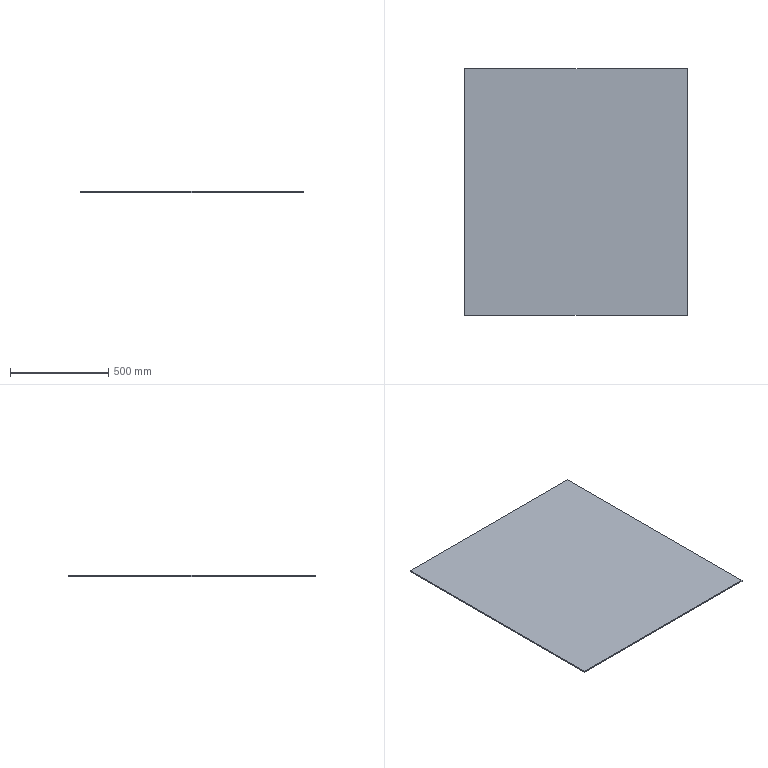Part | SolidWorks | features Extrusion 1 | 1 solid | 6 faces | box 1135 x 1255 x 6 mm | volume 8546550 mm3 | plane 6
STEP:
#1=CARTESIAN_POINT('',(567.5,-627.5,0.));
#2=VERTEX_POINT('',#1);
#3=CARTESIAN_POINT('',(567.5,627.5,0.));
#4=VERTEX_POINT('',#3);
#5=CARTESIAN_POINT('',(567.5,627.5,0.));
#6=DIRECTION('',(0.,1.,0.));
#7=VECTOR('',#6,1000.);
#8=LINE('',#5,#7);
#9=EDGE_CURVE('',#2,#4,#8,.T.);
#10=ORIENTED_EDGE('',*,*,#9,.T.);
#11=CARTESIAN_POINT('',(567.5,627.5,6.));
#12=VERTEX_POINT('',#11);
#13=CARTESIAN_POINT('',(567.5,627.5,6.));
#14=DIRECTION('',(0.,0.,-1.));
#15=VECTOR('',#14,1000.);
#16=LINE('',#13,#15);
#17=EDGE_CURVE('',#12,#4,#16,.T.);
#18=ORIENTED_EDGE('',*,*,#17,.F.);
#19=CARTESIAN_POINT('',(567.5,-627.5,6.));
#20=VERTEX_POINT('',#19);
#21=CARTESIAN_POINT('',(567.5,627.5,6.));
#22=DIRECTION('',(0.,1.,0.));
#23=VECTOR('',#22,1000.);
#24=LINE('',#21,#23);
#25=EDGE_CURVE('',#20,#12,#24,.T.);
#26=ORIENTED_EDGE('',*,*,#25,.F.);
#27=CARTESIAN_POINT('',(567.5,-627.5,6.));
#28=DIRECTION('',(0.,0.,-1.));
#29=VECTOR('',#28,1000.);
#30=LINE('',#27,#29);
#31=EDGE_CURVE('',#20,#2,#30,.T.);
#32=ORIENTED_EDGE('',*,*,#31,.T.);
#33=EDGE_LOOP('',(#10,#18,#26,#32));
#34=FACE_OUTER_BOUND('',#33,.T.);
#35=CARTESIAN_POINT('',(567.5,627.5,6.));
#36=DIRECTION('',(-1.,0.,0.));
#37=DIRECTION('',(0.,-1.,0.));
#38=AXIS2_PLACEMENT_3D('',#35,#36,#37);
#39=PLANE('',#38);
#40=ADVANCED_FACE('',(#34),#39,.F.);
#41=CARTESIAN_POINT('',(-567.5,627.5,0.));
#42=VERTEX_POINT('',#41);
#43=CARTESIAN_POINT('',(-567.5,627.5,0.));
#44=DIRECTION('',(-1.,0.,0.));
#45=VECTOR('',#44,1000.);
#46=LINE('',#43,#45);
#47=EDGE_CURVE('',#4,#42,#46,.T.);
#48=ORIENTED_EDGE('',*,*,#47,.T.);
#49=CARTESIAN_POINT('',(-567.5,627.5,6.));
#50=VERTEX_POINT('',#49);
#51=CARTESIAN_POINT('',(-567.5,627.5,6.));
#52=DIRECTION('',(0.,0.,-1.));
#53=VECTOR('',#52,1000.);
#54=LINE('',#51,#53);
#55=EDGE_CURVE('',#50,#42,#54,.T.);
#56=ORIENTED_EDGE('',*,*,#55,.F.);
#57=CARTESIAN_POINT('',(-567.5,627.5,6.));
#58=DIRECTION('',(-1.,0.,0.));
#59=VECTOR('',#58,1000.);
#60=LINE('',#57,#59);
#61=EDGE_CURVE('',#12,#50,#60,.T.);
#62=ORIENTED_EDGE('',*,*,#61,.F.);
#63=ORIENTED_EDGE('',*,*,#17,.T.);
#64=EDGE_LOOP('',(#48,#56,#62,#63));
#65=FACE_OUTER_BOUND('',#64,.T.);
#66=CARTESIAN_POINT('',(-567.5,627.5,6.));
#67=DIRECTION('',(0.,-1.,0.));
#68=DIRECTION('',(0.,0.,-1.));
#69=AXIS2_PLACEMENT_3D('',#66,#67,#68);
#70=PLANE('',#69);
#71=ADVANCED_FACE('',(#65),#70,.F.);
#72=CARTESIAN_POINT('',(-567.5,-627.5,0.));
#73=VERTEX_POINT('',#72);
#74=CARTESIAN_POINT('',(-567.5,627.5,0.));
#75=DIRECTION('',(0.,-1.,0.));
#76=VECTOR('',#75,1000.);
#77=LINE('',#74,#76);
#78=EDGE_CURVE('',#42,#73,#77,.T.);
#79=ORIENTED_EDGE('',*,*,#78,.T.);
#80=CARTESIAN_POINT('',(-567.5,-627.5,6.));
#81=VERTEX_POINT('',#80);
#82=CARTESIAN_POINT('',(-567.5,-627.5,6.));
#83=DIRECTION('',(0.,0.,-1.));
#84=VECTOR('',#83,1000.);
#85=LINE('',#82,#84);
#86=EDGE_CURVE('',#81,#73,#85,.T.);
#87=ORIENTED_EDGE('',*,*,#86,.F.);
#88=CARTESIAN_POINT('',(-567.5,627.5,6.));
#89=DIRECTION('',(0.,-1.,0.));
#90=VECTOR('',#89,1000.);
#91=LINE('',#88,#90);
#92=EDGE_CURVE('',#50,#81,#91,.T.);
#93=ORIENTED_EDGE('',*,*,#92,.F.);
#94=ORIENTED_EDGE('',*,*,#55,.T.);
#95=EDGE_LOOP('',(#79,#87,#93,#94));
#96=FACE_OUTER_BOUND('',#95,.T.);
#97=CARTESIAN_POINT('',(-567.5,627.5,6.));
#98=DIRECTION('',(1.,0.,0.));
#99=DIRECTION('',(0.,1.,0.));
#100=AXIS2_PLACEMENT_3D('',#97,#98,#99);
#101=PLANE('',#100);
#102=ADVANCED_FACE('',(#96),#101,.F.);
#103=CARTESIAN_POINT('',(-567.5,-627.5,0.));
#104=DIRECTION('',(1.,0.,0.));
#105=VECTOR('',#104,1000.);
#106=LINE('',#103,#105);
#107=EDGE_CURVE('',#73,#2,#106,.T.);
#108=ORIENTED_EDGE('',*,*,#107,.T.);
#109=ORIENTED_EDGE('',*,*,#31,.F.);
#110=CARTESIAN_POINT('',(-567.5,-627.5,6.));
#111=DIRECTION('',(1.,0.,0.));
#112=VECTOR('',#111,1000.);
#113=LINE('',#110,#112);
#114=EDGE_CURVE('',#81,#20,#113,.T.);
#115=ORIENTED_EDGE('',*,*,#114,.F.);
#116=ORIENTED_EDGE('',*,*,#86,.T.);
#117=EDGE_LOOP('',(#108,#109,#115,#116));
#118=FACE_OUTER_BOUND('',#117,.T.);
#119=CARTESIAN_POINT('',(-567.5,-627.5,6.));
#120=DIRECTION('',(0.,1.,0.));
#121=DIRECTION('',(0.,0.,1.));
#122=AXIS2_PLACEMENT_3D('',#119,#120,#121);
#123=PLANE('',#122);
#124=ADVANCED_FACE('',(#118),#123,.F.);
#125=ORIENTED_EDGE('',*,*,#25,.T.);
#126=ORIENTED_EDGE('',*,*,#61,.T.);
#127=ORIENTED_EDGE('',*,*,#92,.T.);
#128=ORIENTED_EDGE('',*,*,#114,.T.);
#129=EDGE_LOOP('',(#125,#126,#127,#128));
#130=FACE_OUTER_BOUND('',#129,.T.);
#131=CARTESIAN_POINT('',(0.,0.,6.));
#132=DIRECTION('',(0.,0.,1.));
#133=DIRECTION('',(1.,0.,0.));
#134=AXIS2_PLACEMENT_3D('',#131,#132,#133);
#135=PLANE('',#134);
#136=ADVANCED_FACE('',(#130),#135,.T.);
#137=ORIENTED_EDGE('',*,*,#9,.F.);
#138=ORIENTED_EDGE('',*,*,#107,.F.);
#139=ORIENTED_EDGE('',*,*,#78,.F.);
#140=ORIENTED_EDGE('',*,*,#47,.F.);
#141=EDGE_LOOP('',(#137,#138,#139,#140));
#142=FACE_OUTER_BOUND('',#141,.T.);
#143=CARTESIAN_POINT('',(0.,0.,0.));
#144=DIRECTION('',(0.,0.,1.));
#145=DIRECTION('',(1.,0.,0.));
#146=AXIS2_PLACEMENT_3D('',#143,#144,#145);
#147=PLANE('',#146);
#148=ADVANCED_FACE('',(#142),#147,.F.);
#149=CLOSED_SHELL('',(#40,#71,#102,#124,#136,#148));
#150=MANIFOLD_SOLID_BREP('',#149);
#151=CARTESIAN_POINT('',(0.,0.,0.));
#152=DIRECTION('',(0.,0.,1.));
#153=DIRECTION('',(1.,0.,0.));
#154=AXIS2_PLACEMENT_3D('',#151,#152,#153);
#155=(LENGTH_UNIT()NAMED_UNIT(*)SI_UNIT(.MILLI.,.METRE.));
#156=UNCERTAINTY_MEASURE_WITH_UNIT(LENGTH_MEASURE(0.00001),#155,'','');
#157=(NAMED_UNIT(*)PLANE_ANGLE_UNIT()SI_UNIT($,.RADIAN.));
#158=(NAMED_UNIT(*)SI_UNIT($,.STERADIAN.)SOLID_ANGLE_UNIT());
#159=(GEOMETRIC_REPRESENTATION_CONTEXT(3)GLOBAL_UNCERTAINTY_ASSIGNED_CONTEXT((#156))GLOBAL_UNIT_ASSIGNED_CONTEXT((#155,#157,#158))REPRESENTATION_CONTEXT('',''));
#160=ADVANCED_BREP_SHAPE_REPRESENTATION('',(#150,#154),#159);